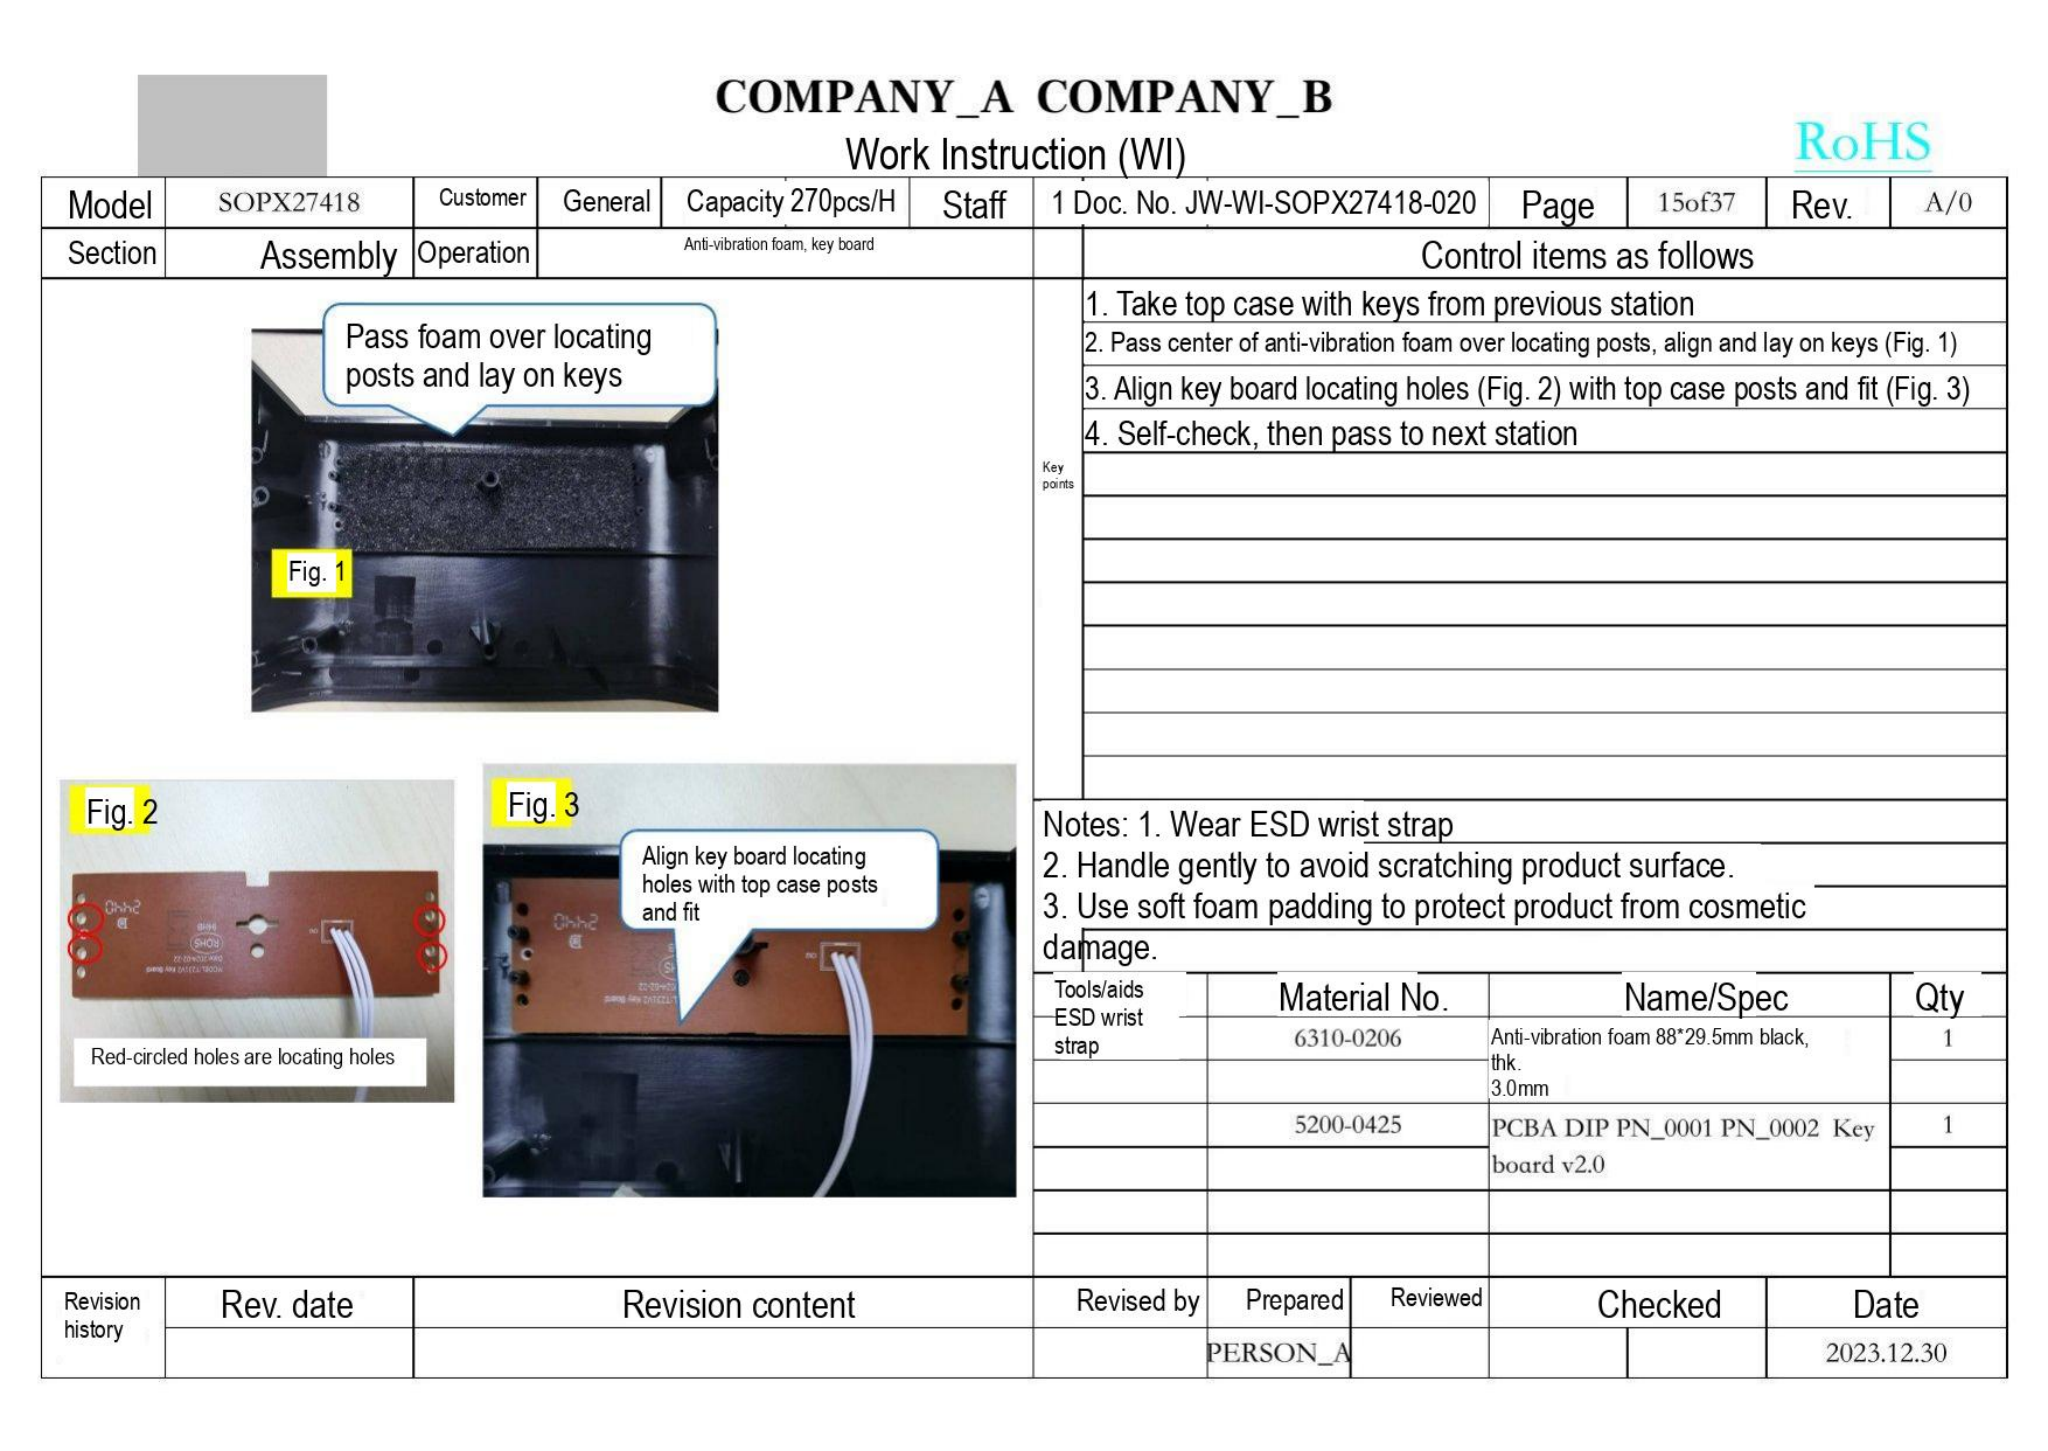COMPANY_A COMPANY_B

Work Instruction (WI)

RoHS

| Model | SOPX27418 | Customer | General | Capacity 270pcs/H | Staff | 1 Doc. No. JW-WI-SOPX27418-020 | Page | 15of37 | Rev. | A/0 |
|---|---|---|---|---|---|---|---|---|---|---|
| Section | Assembly | Operation | Anti-vibration foam, key board | | | | | | | |

Pass foam over locating posts and lay on keys

Fig. 1

Fig. 2

Red-circled holes are locating holes

Fig. 3

Align key board locating holes with top case posts and fit

Control items as follows

| Key points | |
|---|---|
| | 1. Take top case with keys from previous station |
| | 2. Pass center of anti-vibration foam over locating posts, align and lay on keys (Fig. 1) |
| | 3. Align key board locating holes (Fig. 2) with top case posts and fit (Fig. 3) |
| | 4. Self-check, then pass to next station |

Notes: 1. Wear ESD wrist strap
2. Handle gently to avoid scratching product surface.
3. Use soft foam padding to protect product from cosmetic damage.

| Tools/aids | Material No. | Name/Spec | Qty |
|---|---|---|---|
| ESD wrist strap | 6310-0206 | Anti-vibration foam 88*29.5mm black, thk. 3.0mm | 1 |
| | 5200-0425 | PCBA DIP PN_0001 PN_0002 Key board v2.0 | 1 |

| Revision history | Rev. date | Revision content | Revised by | Prepared | Reviewed | Checked | Date |
|---|---|---|---|---|---|---|---|
| | | | | PERSON_A | | | 2023.12.30 |
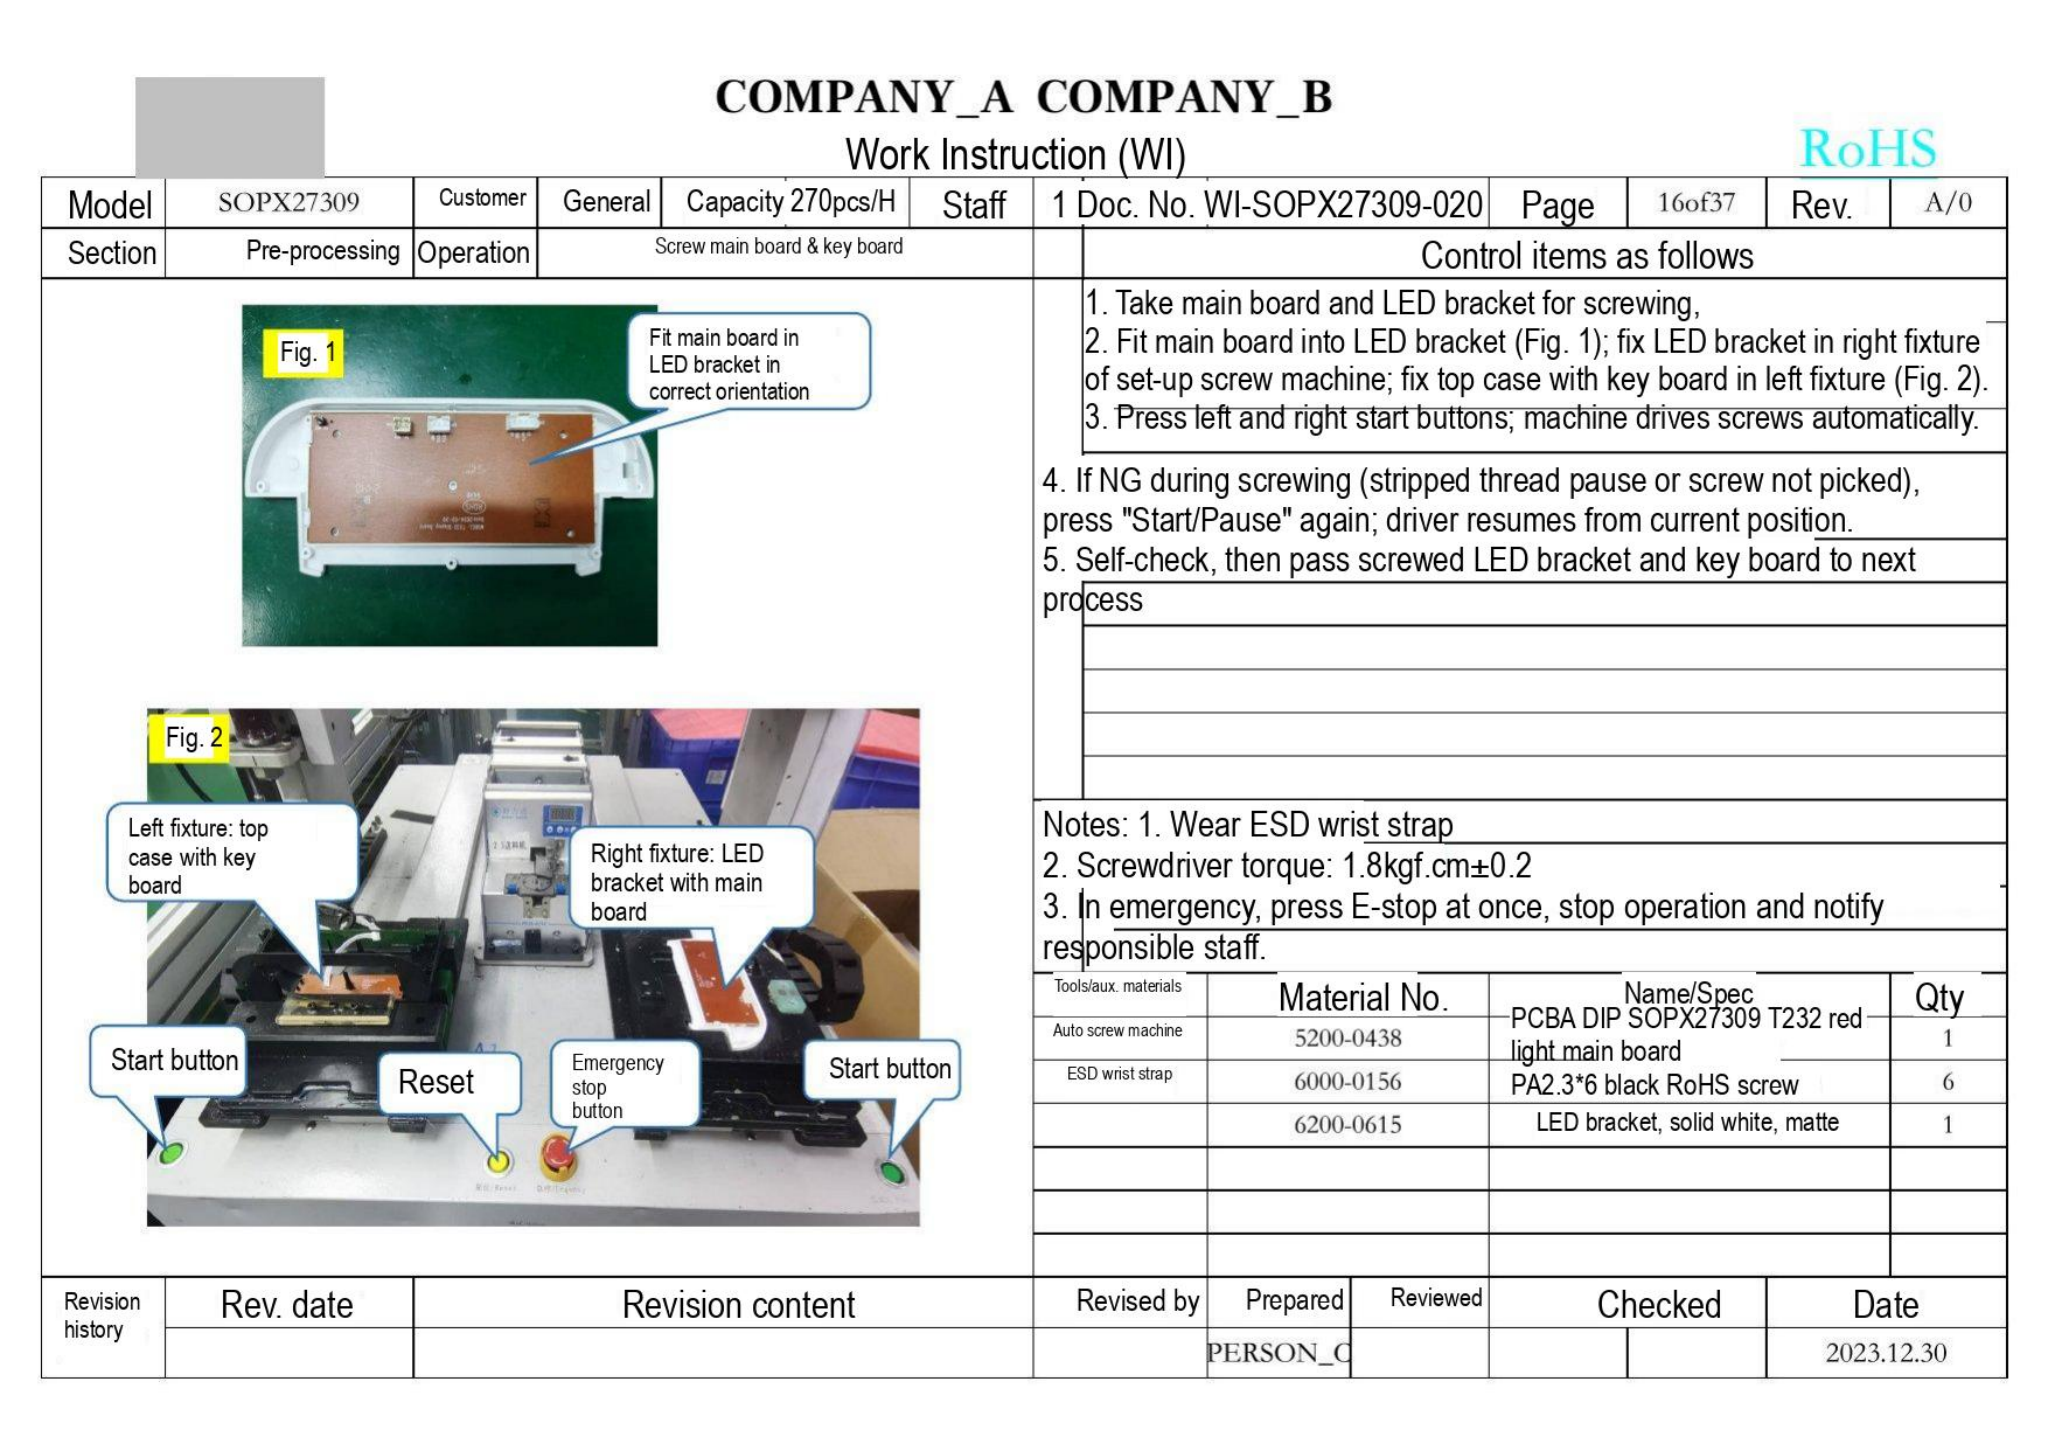COMPANY_A COMPANY_B

Work Instruction (WI)

RoHS

| Model | SOPX27309 | Customer | General | Capacity 270pcs/H | Staff | 1 | Doc. No. WI-SOPX27309-020 | Page | 16of37 | Rev. | A/0 |
|---|---|---|---|---|---|---|---|---|---|---|---|
| Section | Pre-processing | Operation | Screw main board & key board | | | | | | | | |

Fig. 1

Fit main board in LED bracket in correct orientation

Fig. 2

Left fixture: top case with key board

Right fixture: LED bracket with main board

Start button

Reset

Emergency stop button

Start button

Control items as follows

1. Take main board and LED bracket for screwing,
2. Fit main board into LED bracket (Fig. 1); fix LED bracket in right fixture of set-up screw machine; fix top case with key board in left fixture (Fig. 2).
3. Press left and right start buttons; machine drives screws automatically.
4. If NG during screwing (stripped thread pause or screw not picked), press "Start/Pause" again; driver resumes from current position.
5. Self-check, then pass screwed LED bracket and key board to next process

Notes: 1. Wear ESD wrist strap
2. Screwdriver torque: 1.8kgf.cm±0.2
3. In emergency, press E-stop at once, stop operation and notify responsible staff.

| Tools/aux. materials | Material No. | Name/Spec | Qty |
|---|---|---|---|
| Auto screw machine | 5200-0438 | PCBA DIP SOPX27309 T232 red light main board | 1 |
| ESD wrist strap | 6000-0156 | PA2.3*6 black RoHS screw | 6 |
| | 6200-0615 | LED bracket, solid white, matte | 1 |
| | | | |
| | | | |
| | | | |

| Revision history | Rev. date | Revision content | Revised by | Prepared | Reviewed | Checked | Date |
|---|---|---|---|---|---|---|---|
| | | | | PERSON_C | | | 2023.12.30 |
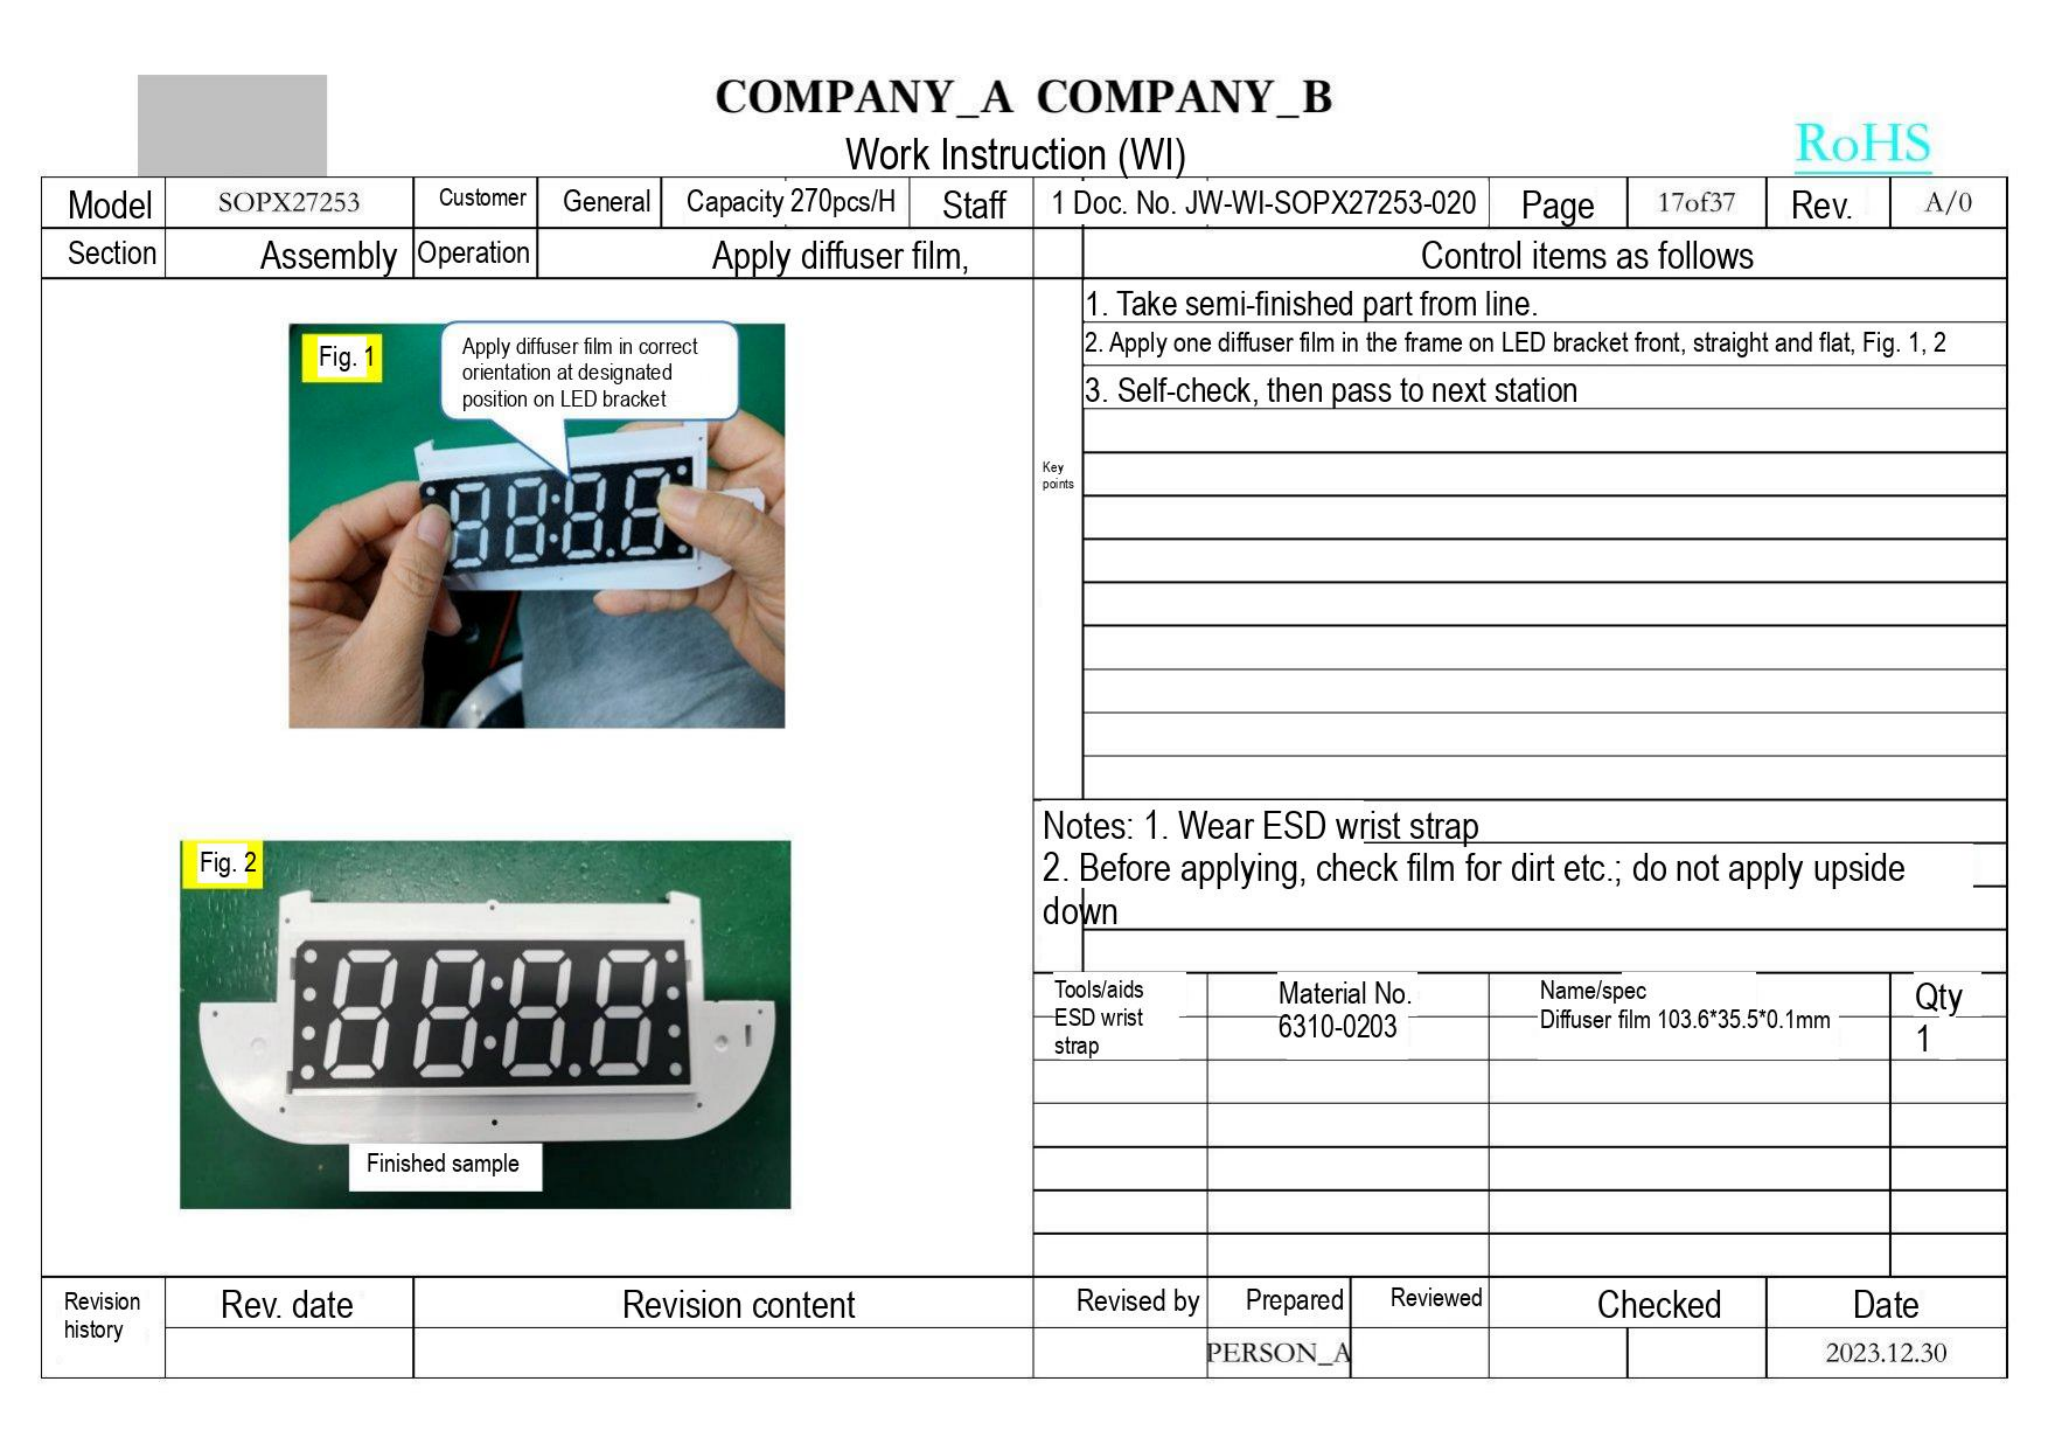COMPANY_A COMPANY_B
Work Instruction (WI)
RoHS

| Model | SOPX27253 | Customer | General | Capacity 270pcs/H | Staff | 1 Doc. No. JW-WI-SOPX27253-020 | Page | 17of37 | Rev. | A/0 |
|---|---|---|---|---|---|---|---|---|---|---|
| Section | Assembly | Operation | Apply diffuser film, | | | | | | | |

Control items as follows

1. Take semi-finished part from line.
2. Apply one diffuser film in the frame on LED bracket front, straight and flat, Fig. 1, 2
3. Self-check, then pass to next station

Key points

Fig. 1
Apply diffuser film in correct orientation at designated position on LED bracket

Fig. 2
Finished sample

Notes: 1. Wear ESD wrist strap
2. Before applying, check film for dirt etc.; do not apply upside down

| Tools/aids | Material No. | Name/spec | Qty |
|---|---|---|---|
| ESD wrist strap | 6310-0203 | Diffuser film 103.6*35.5*0.1mm | 1 |

| Revision history | Rev. date | Revision content | Revised by | Prepared | Reviewed | Checked | Date |
|---|---|---|---|---|---|---|---|
| | | | | PERSON_A | | | 2023.12.30 |
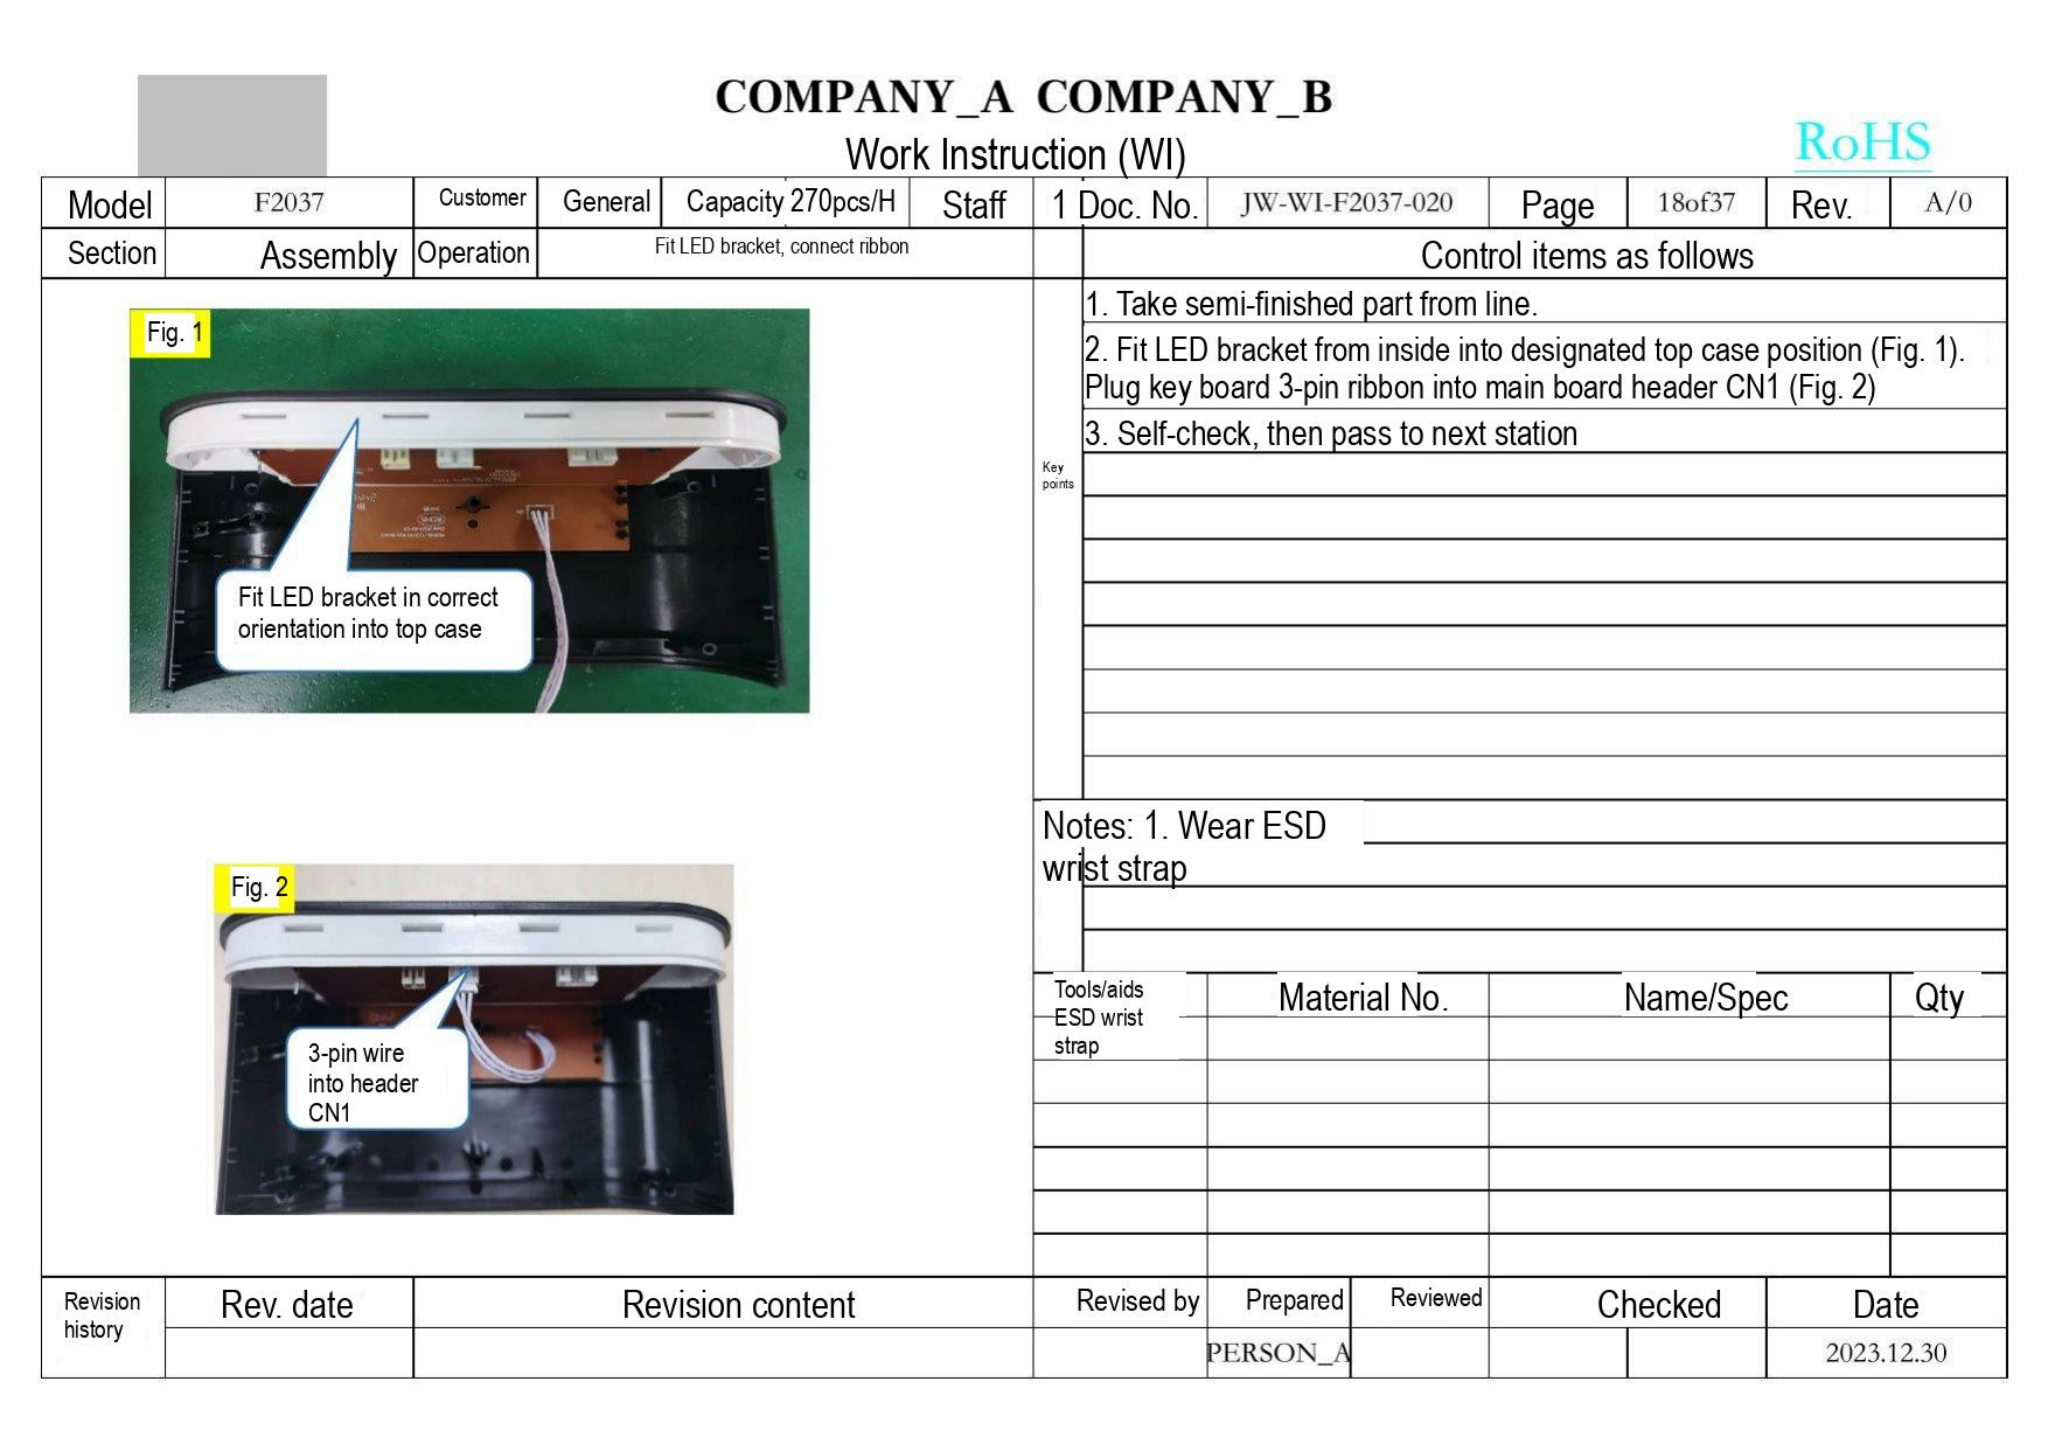COMPANY_A COMPANY_B

Work Instruction (WI)

RoHS

| Model | F2037 | Customer | General | Capacity 270pcs/H | Staff | 1 | Doc. No. | JW-WI-F2037-020 | Page | 18of37 | Rev. | A/0 |
|---|---|---|---|---|---|---|---|---|---|---|---|---|
| Section | Assembly | Operation | Fit LED bracket, connect ribbon | | | | | | | | | |

Fig. 1

Fit LED bracket in correct orientation into top case

Fig. 2

3-pin wire into header CN1

Control items as follows

| Key points | |
|---|---|
| | 1. Take semi-finished part from line. |
| | 2. Fit LED bracket from inside into designated top case position (Fig. 1). Plug key board 3-pin ribbon into main board header CN1 (Fig. 2) |
| | 3. Self-check, then pass to next station |

Notes: 1. Wear ESD wrist strap

| Tools/aids | Material No. | Name/Spec | Qty |
|---|---|---|---|
| ESD wrist strap | | | |

| Revision history | Rev. date | Revision content | Revised by | Prepared | Reviewed | Checked | Date |
|---|---|---|---|---|---|---|---|
| | | | | PERSON_A | | | 2023.12.30 |
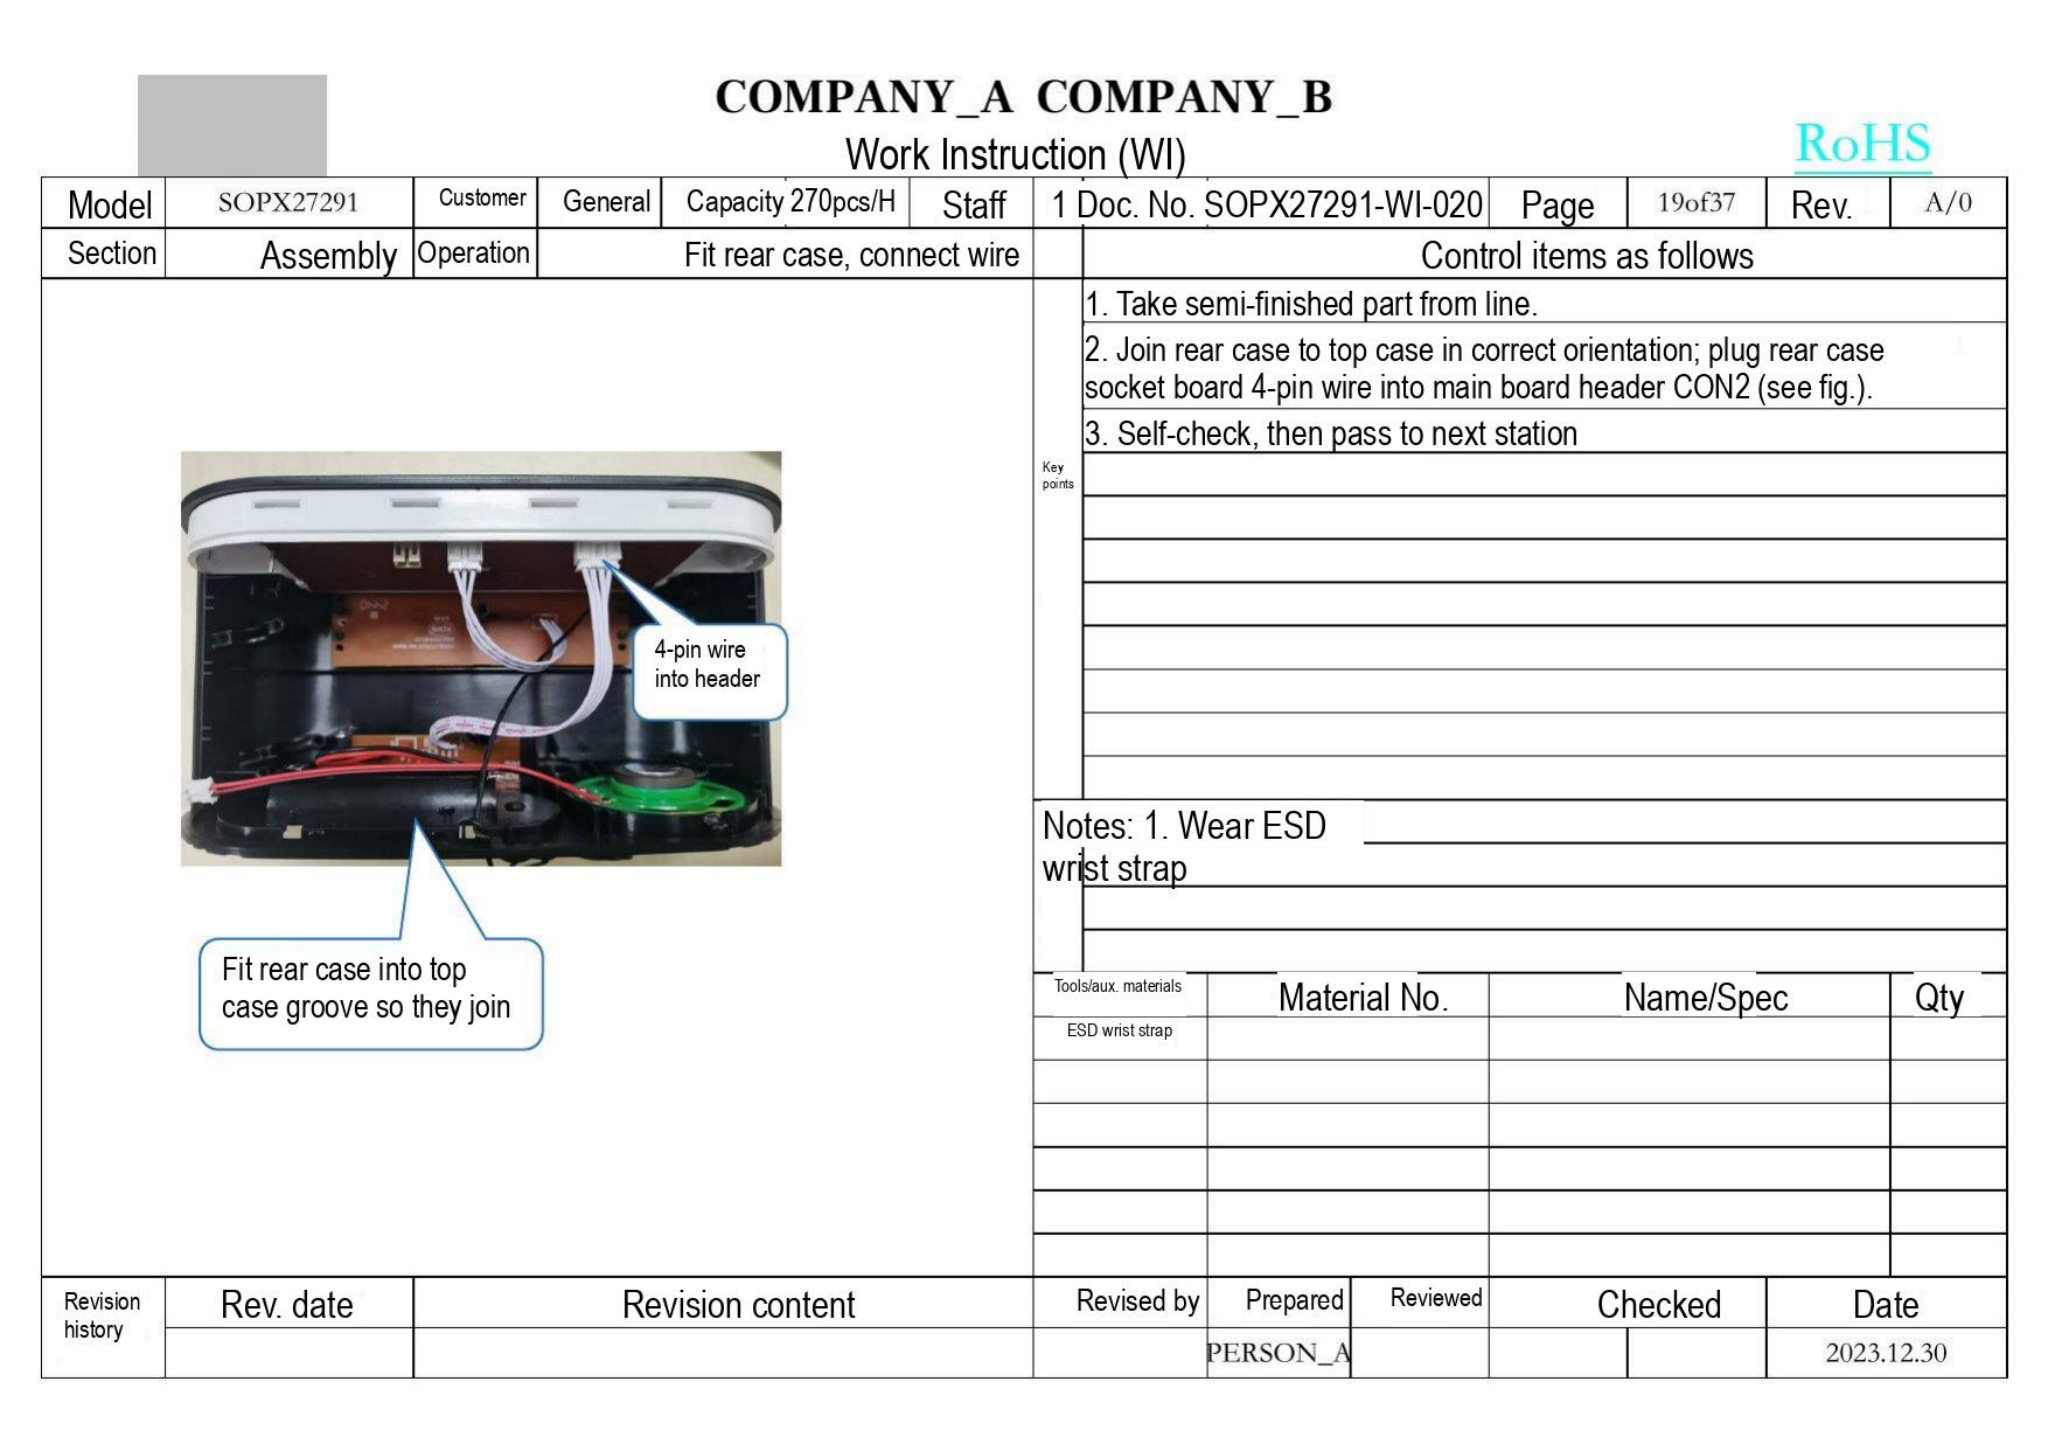COMPANY_A COMPANY_B
Work Instruction (WI)
RoHS

| Model | SOPX27291 | Customer | General | Capacity 270pcs/H | Staff | 1 Doc. No. SOPX27291-WI-020 | Page | 19of37 | Rev. | A/0 |
|---|---|---|---|---|---|---|---|---|---|---|
| Section | Assembly | Operation | Fit rear case, connect wire | | | | | | | |

4-pin wire into header

Fit rear case into top case groove so they join

| Key points | Control items as follows |
|---|---|
| | 1. Take semi-finished part from line. |
| | 2. Join rear case to top case in correct orientation; plug rear case socket board 4-pin wire into main board header CON2 (see fig.). |
| | 3. Self-check, then pass to next station |

Notes: 1. Wear ESD wrist strap

| Tools/aux. materials | Material No. | Name/Spec | Qty |
|---|---|---|---|
| ESD wrist strap | | | |

| Revision history | Rev. date | Revision content | Revised by | Prepared | Reviewed | Checked | Date |
|---|---|---|---|---|---|---|---|
| | | | | PERSON_A | | | 2023.12.30 |
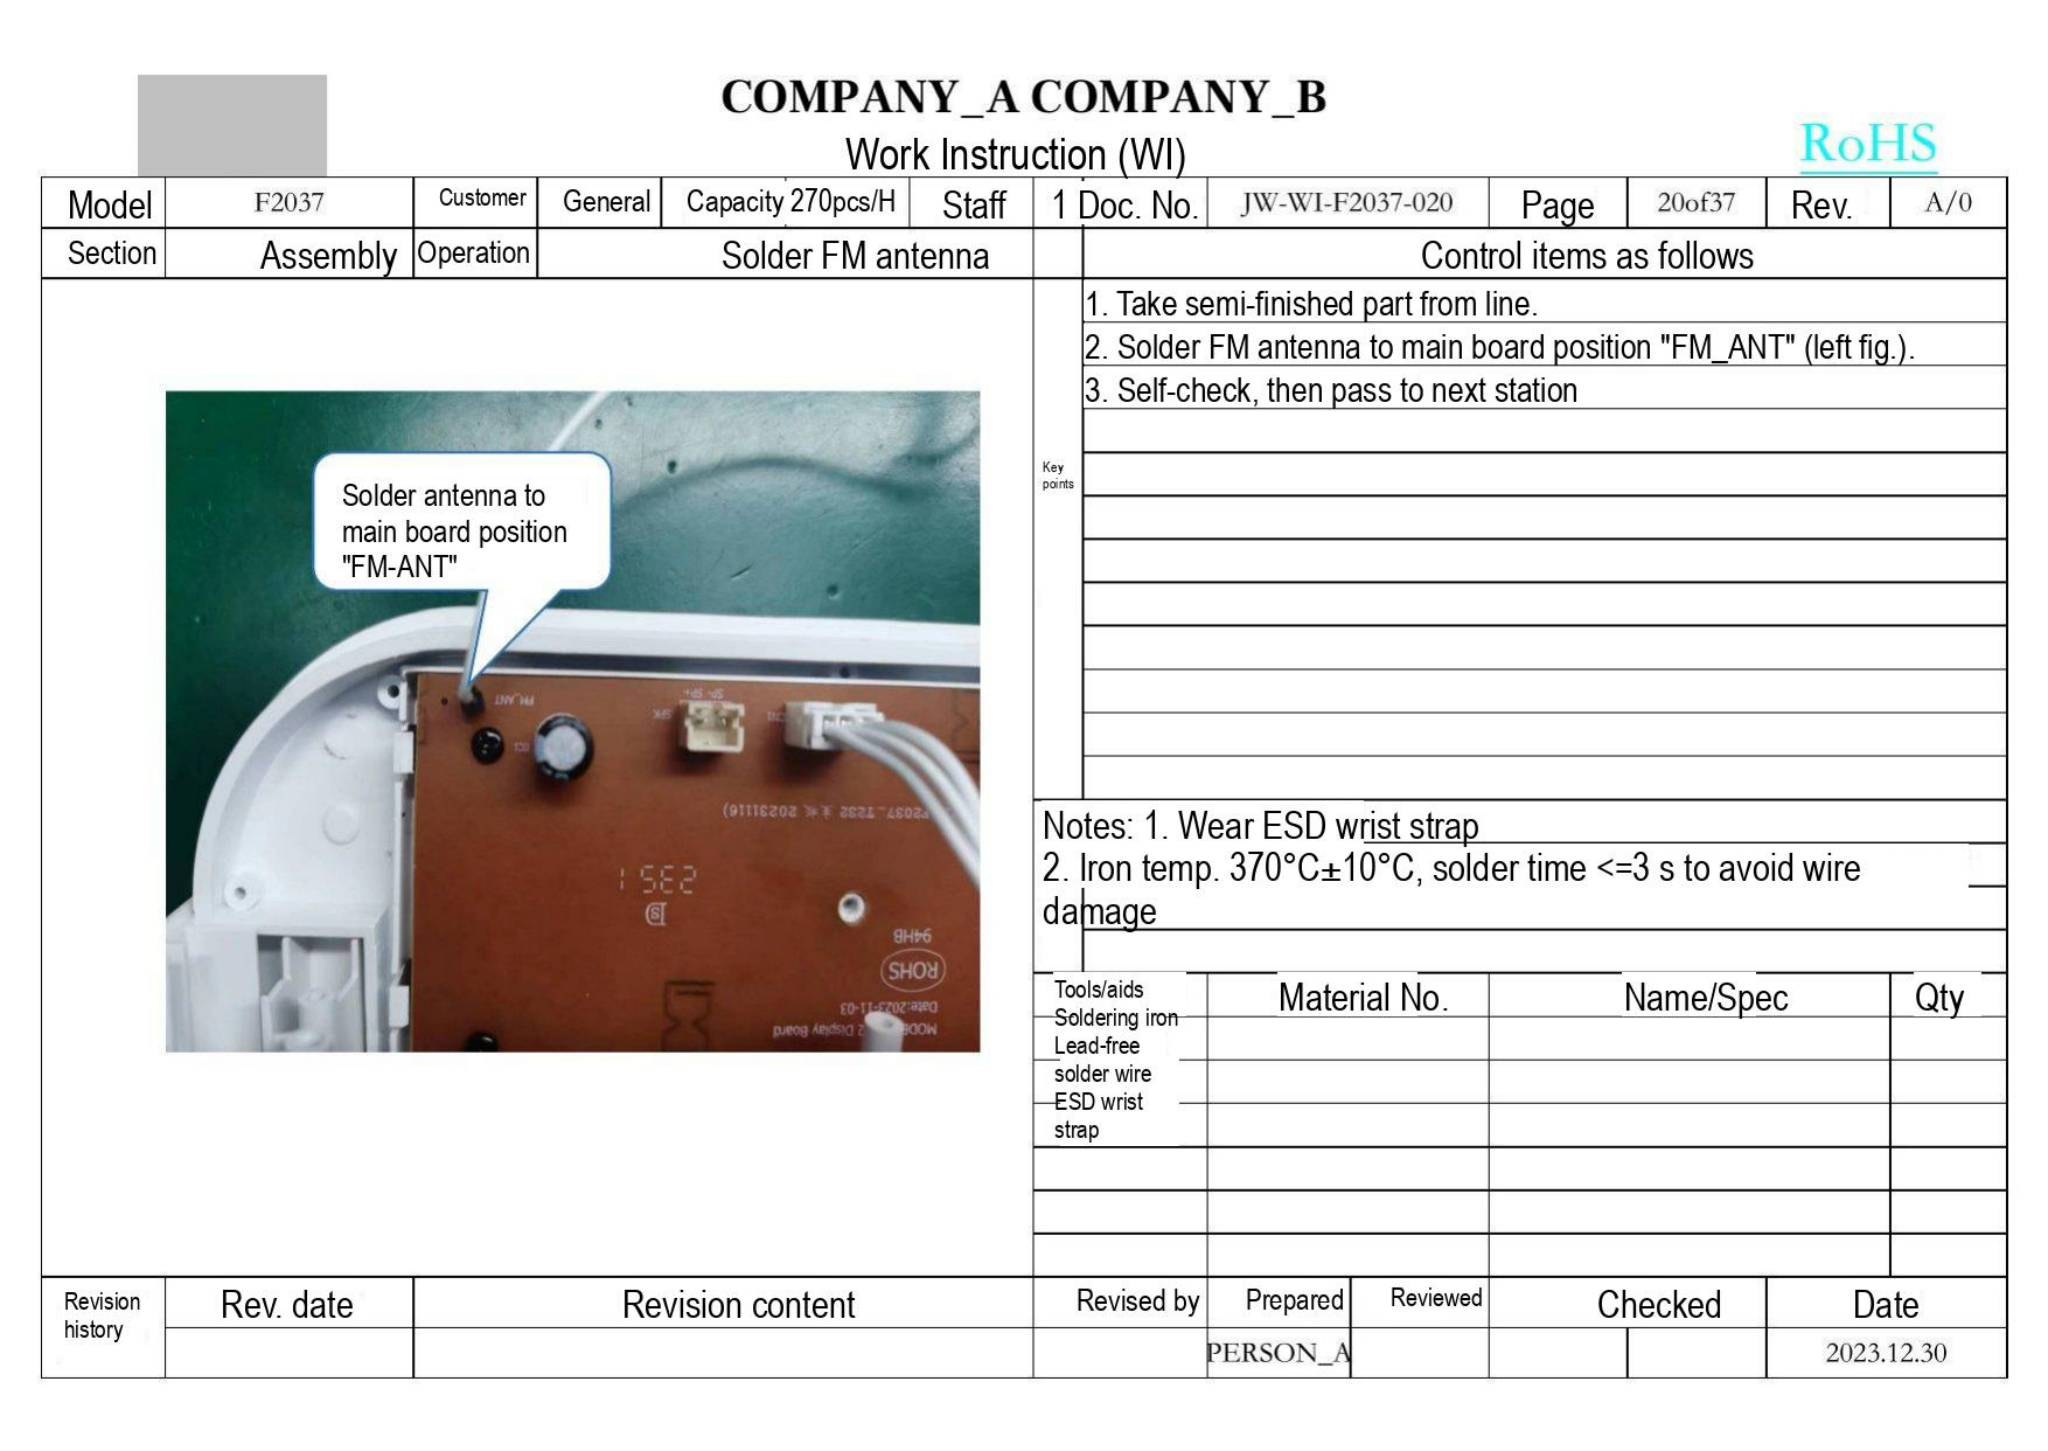COMPANY_A COMPANY_B
Work Instruction (WI)
RoHS

| Model | F2037 | Customer | General | Capacity 270pcs/H | Staff | 1 | Doc. No. | JW-WI-F2037-020 | Page | 20of37 | Rev. | A/0 |
|---|---|---|---|---|---|---|---|---|---|---|---|---|
| Section | Assembly | Operation | Solder FM antenna | | | | | | | | | |

Solder antenna to main board position "FM-ANT"

FM_ANT
SP- SP+
SPK
CN1
C1
F2037_T232 ✱✱ 20231116
1 S32
94HB
ROHS
Date:2023-11-03
MODEL 2 Display Board

Control items as follows

Key points
1. Take semi-finished part from line.
2. Solder FM antenna to main board position "FM_ANT" (left fig.).
3. Self-check, then pass to next station

Notes: 1. Wear ESD wrist strap
2. Iron temp. 370°C±10°C, solder time <=3 s to avoid wire damage

| Tools/aids | Material No. | Name/Spec | Qty |
|---|---|---|---|
| Soldering iron<br>Lead-free solder wire<br>ESD wrist strap | | | |

| Revision history | Rev. date | Revision content | Revised by | Prepared | Reviewed | Checked | Date |
|---|---|---|---|---|---|---|---|
| | | | | PERSON_A | | | 2023.12.30 |
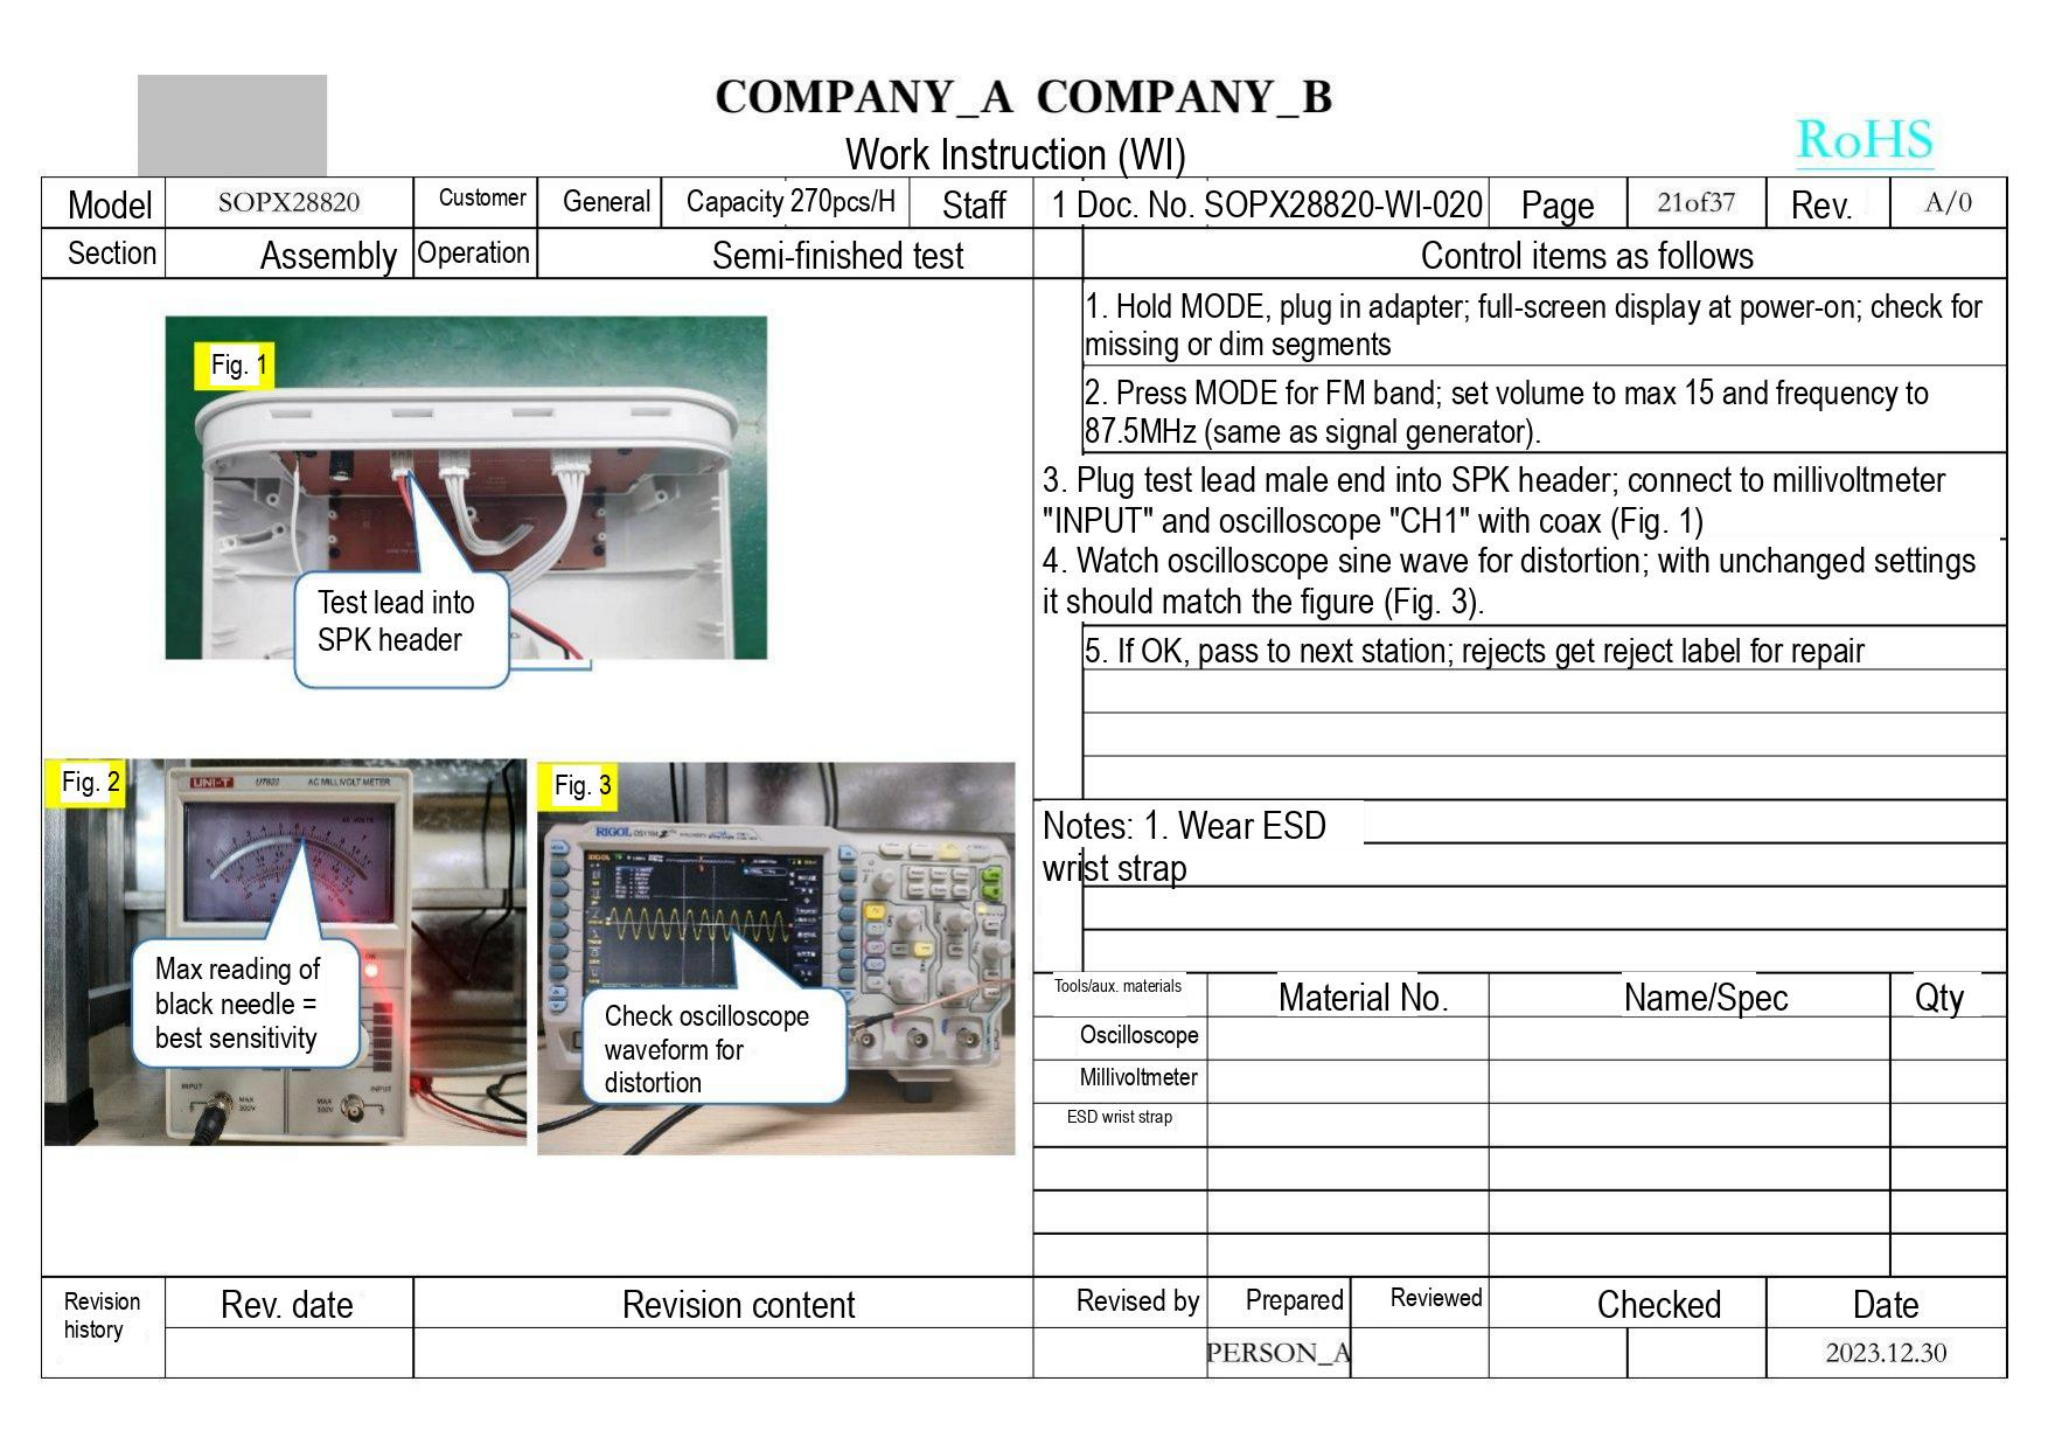COMPANY_A COMPANY_B
Work Instruction (WI)
RoHS

| Model | SOPX28820 | Customer | General | Capacity 270pcs/H | Staff | 1 Doc. No. SOPX28820-WI-020 | Page | 21of37 | Rev. | A/0 |
|---|---|---|---|---|---|---|---|---|---|---|
| Section | Assembly | Operation | Semi-finished test | | | Control items as follows | | | | |

Fig. 1
Test lead into SPK header

Fig. 2
UNI-T UT632 AC MILLIVOLT METER
Max reading of black needle = best sensitivity
INPUT MAX 300V
MAX 300V INPUT

Fig. 3
RIGOL DS1104Z
Check oscilloscope waveform for distortion

Control items as follows
1. Hold MODE, plug in adapter; full-screen display at power-on; check for missing or dim segments
2. Press MODE for FM band; set volume to max 15 and frequency to 87.5MHz (same as signal generator).
3. Plug test lead male end into SPK header; connect to millivoltmeter "INPUT" and oscilloscope "CH1" with coax (Fig. 1)
4. Watch oscilloscope sine wave for distortion; with unchanged settings it should match the figure (Fig. 3).
5. If OK, pass to next station; rejects get reject label for repair

Notes: 1. Wear ESD wrist strap

| Tools/aux. materials | Material No. | Name/Spec | Qty |
|---|---|---|---|
| Oscilloscope | | | |
| Millivoltmeter | | | |
| ESD wrist strap | | | |
| | | | |
| | | | |
| | | | |

| Revision history | Rev. date | Revision content | Revised by | Prepared | Reviewed | Checked | Date |
|---|---|---|---|---|---|---|---|
| | | | | PERSON_A | | | 2023.12.30 |